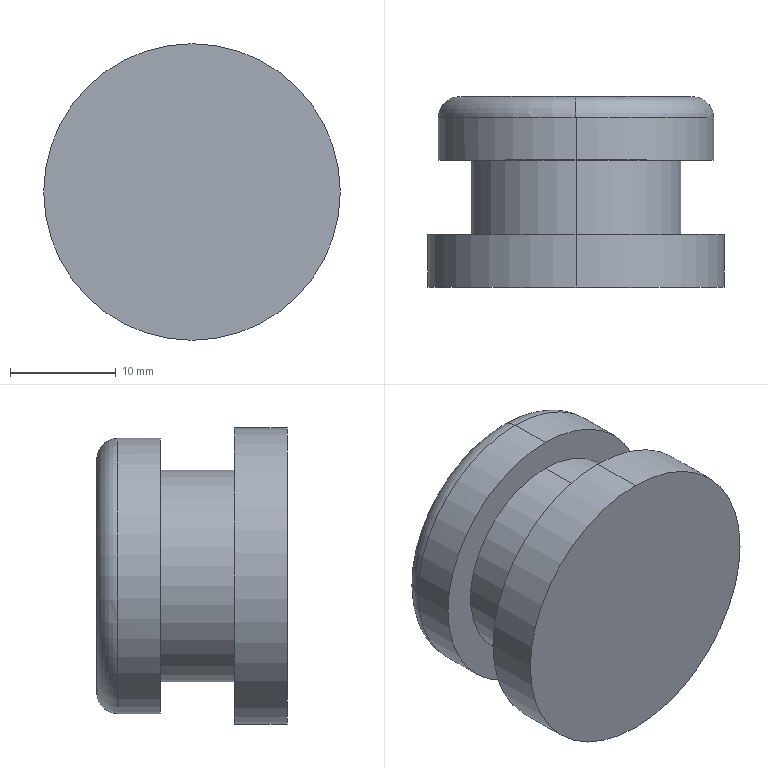Part | NX | features solid 2 | 1 solid | 12 faces | box 28 x 18 x 28 mm | volume 8396 mm3 | cylinder 6 | plane 4 | torus 2 | commonest cylinder face diameters 20 x2 26 x2 28 x2
STEP:
#1=CARTESIAN_POINT('',(-190.,-22.1,-151.));
#2=VERTEX_POINT('',#1);
#3=CARTESIAN_POINT('',(-190.,-22.1,-123.));
#4=VERTEX_POINT('',#3);
#5=CARTESIAN_POINT('',(-190.,-22.1,-137.));
#6=DIRECTION('',(0.,-1.,0.));
#7=DIRECTION('',(0.,0.,-1.));
#8=AXIS2_PLACEMENT_3D('',#5,#6,#7);
#9=CIRCLE('',#8,14.);
#10=EDGE_CURVE('',#2,#4,#9,.T.);
#11=ORIENTED_EDGE('',*,*,#10,.T.);
#12=CARTESIAN_POINT('',(-190.,-27.1,-123.));
#13=VERTEX_POINT('',#12);
#14=CARTESIAN_POINT('',(-190.,-27.1,-123.));
#15=DIRECTION('',(0.,1.,0.));
#16=VECTOR('',#15,1000.);
#17=LINE('',#14,#16);
#18=EDGE_CURVE('',#13,#4,#17,.T.);
#19=ORIENTED_EDGE('',*,*,#18,.F.);
#20=CARTESIAN_POINT('',(-190.,-27.1,-151.));
#21=VERTEX_POINT('',#20);
#22=CARTESIAN_POINT('',(-190.,-27.1,-137.));
#23=DIRECTION('',(0.,1.,0.));
#24=DIRECTION('',(0.,0.,1.));
#25=AXIS2_PLACEMENT_3D('',#22,#23,#24);
#26=CIRCLE('',#25,14.);
#27=EDGE_CURVE('',#13,#21,#26,.T.);
#28=ORIENTED_EDGE('',*,*,#27,.T.);
#29=CARTESIAN_POINT('',(-190.,-27.1,-151.));
#30=DIRECTION('',(0.,1.,0.));
#31=VECTOR('',#30,1000.);
#32=LINE('',#29,#31);
#33=EDGE_CURVE('',#2,#21,#32,.F.);
#34=ORIENTED_EDGE('',*,*,#33,.F.);
#35=EDGE_LOOP('',(#11,#19,#28,#34));
#36=FACE_BOUND('',#35,.T.);
#37=CARTESIAN_POINT('',(-190.,-21.85,-137.));
#38=DIRECTION('',(0.,-1.,0.));
#39=DIRECTION('',(0.,0.,-1.));
#40=AXIS2_PLACEMENT_3D('',#37,#38,#39);
#41=CYLINDRICAL_SURFACE('',#40,14.);
#42=ADVANCED_FACE('',(#36),#41,.T.);
#43=ORIENTED_EDGE('',*,*,#33,.T.);
#44=CARTESIAN_POINT('',(-190.,-27.1,-137.));
#45=DIRECTION('',(0.,1.,0.));
#46=DIRECTION('',(0.,0.,-1.));
#47=AXIS2_PLACEMENT_3D('',#44,#45,#46);
#48=CIRCLE('',#47,14.);
#49=EDGE_CURVE('',#21,#13,#48,.T.);
#50=ORIENTED_EDGE('',*,*,#49,.T.);
#51=ORIENTED_EDGE('',*,*,#18,.T.);
#52=CARTESIAN_POINT('',(-190.,-22.1,-137.));
#53=DIRECTION('',(0.,-1.,0.));
#54=DIRECTION('',(0.,0.,1.));
#55=AXIS2_PLACEMENT_3D('',#52,#53,#54);
#56=CIRCLE('',#55,14.);
#57=EDGE_CURVE('',#4,#2,#56,.T.);
#58=ORIENTED_EDGE('',*,*,#57,.T.);
#59=EDGE_LOOP('',(#43,#50,#51,#58));
#60=FACE_BOUND('',#59,.T.);
#61=CARTESIAN_POINT('',(-190.,-21.85,-137.));
#62=DIRECTION('',(0.,-1.,0.));
#63=DIRECTION('',(0.,0.,-1.));
#64=AXIS2_PLACEMENT_3D('',#61,#62,#63);
#65=CYLINDRICAL_SURFACE('',#64,14.);
#66=ADVANCED_FACE('',(#60),#65,.T.);
#67=ORIENTED_EDGE('',*,*,#10,.F.);
#68=ORIENTED_EDGE('',*,*,#57,.F.);
#69=EDGE_LOOP('',(#67,#68));
#70=FACE_BOUND('',#69,.T.);
#71=CARTESIAN_POINT('',(-190.,-22.1,-147.));
#72=VERTEX_POINT('',#71);
#73=CARTESIAN_POINT('',(-190.,-22.1,-127.));
#74=VERTEX_POINT('',#73);
#75=CARTESIAN_POINT('',(-190.,-22.1,-137.));
#76=DIRECTION('',(0.,1.,0.));
#77=DIRECTION('',(0.,0.,-1.));
#78=AXIS2_PLACEMENT_3D('',#75,#76,#77);
#79=CIRCLE('',#78,10.);
#80=EDGE_CURVE('',#72,#74,#79,.T.);
#81=ORIENTED_EDGE('',*,*,#80,.F.);
#82=CARTESIAN_POINT('',(-190.,-22.1,-137.));
#83=DIRECTION('',(0.,1.,0.));
#84=DIRECTION('',(0.,0.,1.));
#85=AXIS2_PLACEMENT_3D('',#82,#83,#84);
#86=CIRCLE('',#85,10.);
#87=EDGE_CURVE('',#74,#72,#86,.T.);
#88=ORIENTED_EDGE('',*,*,#87,.F.);
#89=EDGE_LOOP('',(#81,#88));
#90=FACE_BOUND('',#89,.T.);
#91=CARTESIAN_POINT('',(-190.,-22.1,-137.));
#92=DIRECTION('',(0.,-1.,0.));
#93=DIRECTION('',(0.,0.,-1.));
#94=AXIS2_PLACEMENT_3D('',#91,#92,#93);
#95=PLANE('',#94);
#96=ADVANCED_FACE('',(#70,#90),#95,.F.);
#97=CARTESIAN_POINT('',(-190.,-15.1,-147.));
#98=VERTEX_POINT('',#97);
#99=CARTESIAN_POINT('',(-190.,-15.1,-127.));
#100=VERTEX_POINT('',#99);
#101=CARTESIAN_POINT('',(-190.,-15.1,-137.));
#102=DIRECTION('',(0.,-1.,0.));
#103=DIRECTION('',(0.,0.,-1.));
#104=AXIS2_PLACEMENT_3D('',#101,#102,#103);
#105=CIRCLE('',#104,10.);
#106=EDGE_CURVE('',#98,#100,#105,.T.);
#107=ORIENTED_EDGE('',*,*,#106,.T.);
#108=CARTESIAN_POINT('',(-190.,-22.1,-127.));
#109=DIRECTION('',(0.,1.,0.));
#110=VECTOR('',#109,1000.);
#111=LINE('',#108,#110);
#112=EDGE_CURVE('',#100,#74,#111,.F.);
#113=ORIENTED_EDGE('',*,*,#112,.T.);
#114=ORIENTED_EDGE('',*,*,#87,.T.);
#115=CARTESIAN_POINT('',(-190.,-22.1,-147.));
#116=DIRECTION('',(0.,1.,0.));
#117=VECTOR('',#116,1000.);
#118=LINE('',#115,#117);
#119=EDGE_CURVE('',#72,#98,#118,.T.);
#120=ORIENTED_EDGE('',*,*,#119,.T.);
#121=EDGE_LOOP('',(#107,#113,#114,#120));
#122=FACE_BOUND('',#121,.T.);
#123=CARTESIAN_POINT('',(-190.,-15.1,-137.));
#124=DIRECTION('',(0.,-1.,0.));
#125=DIRECTION('',(0.,0.,-1.));
#126=AXIS2_PLACEMENT_3D('',#123,#124,#125);
#127=CYLINDRICAL_SURFACE('',#126,10.);
#128=ADVANCED_FACE('',(#122),#127,.T.);
#129=ORIENTED_EDGE('',*,*,#119,.F.);
#130=ORIENTED_EDGE('',*,*,#80,.T.);
#131=ORIENTED_EDGE('',*,*,#112,.F.);
#132=CARTESIAN_POINT('',(-190.,-15.1,-137.));
#133=DIRECTION('',(0.,-1.,0.));
#134=DIRECTION('',(0.,0.,1.));
#135=AXIS2_PLACEMENT_3D('',#132,#133,#134);
#136=CIRCLE('',#135,10.);
#137=EDGE_CURVE('',#100,#98,#136,.T.);
#138=ORIENTED_EDGE('',*,*,#137,.T.);
#139=EDGE_LOOP('',(#129,#130,#131,#138));
#140=FACE_BOUND('',#139,.T.);
#141=CARTESIAN_POINT('',(-190.,-15.1,-137.));
#142=DIRECTION('',(0.,-1.,0.));
#143=DIRECTION('',(0.,0.,-1.));
#144=AXIS2_PLACEMENT_3D('',#141,#142,#143);
#145=CYLINDRICAL_SURFACE('',#144,10.);
#146=ADVANCED_FACE('',(#140),#145,.T.);
#147=CARTESIAN_POINT('',(-190.,-15.1,-124.));
#148=VERTEX_POINT('',#147);
#149=CARTESIAN_POINT('',(-190.,-15.1,-150.));
#150=VERTEX_POINT('',#149);
#151=CARTESIAN_POINT('',(-190.,-15.1,-137.));
#152=DIRECTION('',(0.,1.,0.));
#153=DIRECTION('',(0.,0.,1.));
#154=AXIS2_PLACEMENT_3D('',#151,#152,#153);
#155=CIRCLE('',#154,13.);
#156=EDGE_CURVE('',#148,#150,#155,.T.);
#157=ORIENTED_EDGE('',*,*,#156,.F.);
#158=CARTESIAN_POINT('',(-190.,-15.1,-137.));
#159=DIRECTION('',(0.,1.,0.));
#160=DIRECTION('',(0.,0.,-1.));
#161=AXIS2_PLACEMENT_3D('',#158,#159,#160);
#162=CIRCLE('',#161,13.);
#163=EDGE_CURVE('',#150,#148,#162,.T.);
#164=ORIENTED_EDGE('',*,*,#163,.F.);
#165=EDGE_LOOP('',(#157,#164));
#166=FACE_BOUND('',#165,.T.);
#167=ORIENTED_EDGE('',*,*,#106,.F.);
#168=ORIENTED_EDGE('',*,*,#137,.F.);
#169=EDGE_LOOP('',(#167,#168));
#170=FACE_BOUND('',#169,.T.);
#171=CARTESIAN_POINT('',(-190.,-15.1,-137.));
#172=DIRECTION('',(0.,-1.,0.));
#173=DIRECTION('',(0.,0.,-1.));
#174=AXIS2_PLACEMENT_3D('',#171,#172,#173);
#175=PLANE('',#174);
#176=ADVANCED_FACE('',(#166,#170),#175,.T.);
#177=CARTESIAN_POINT('',(-190.089,-11.1,-124.));
#178=VERTEX_POINT('',#177);
#179=CARTESIAN_POINT('',(-190.,-11.1,-150.));
#180=VERTEX_POINT('',#179);
#181=CARTESIAN_POINT('',(-190.,-11.1,-137.));
#182=DIRECTION('',(0.,-1.,0.));
#183=DIRECTION('',(-0.006879,0.,1.));
#184=AXIS2_PLACEMENT_3D('',#181,#182,#183);
#185=CIRCLE('',#184,13.);
#186=EDGE_CURVE('',#178,#180,#185,.T.);
#187=ORIENTED_EDGE('',*,*,#186,.T.);
#188=CARTESIAN_POINT('',(-190.,-15.1,-150.));
#189=DIRECTION('',(0.,1.,0.));
#190=VECTOR('',#189,1000.);
#191=LINE('',#188,#190);
#192=EDGE_CURVE('',#180,#150,#191,.F.);
#193=ORIENTED_EDGE('',*,*,#192,.T.);
#194=ORIENTED_EDGE('',*,*,#163,.T.);
#195=CARTESIAN_POINT('',(-190.,-11.1,-124.));
#196=VERTEX_POINT('',#195);
#197=CARTESIAN_POINT('',(-190.,-15.1,-124.));
#198=DIRECTION('',(0.,1.,0.));
#199=VECTOR('',#198,1000.);
#200=LINE('',#197,#199);
#201=EDGE_CURVE('',#148,#196,#200,.T.);
#202=ORIENTED_EDGE('',*,*,#201,.T.);
#203=CARTESIAN_POINT('',(-190.,-11.1,-137.));
#204=DIRECTION('',(0.,-1.,0.));
#205=DIRECTION('',(0.,0.,1.));
#206=AXIS2_PLACEMENT_3D('',#203,#204,#205);
#207=CIRCLE('',#206,13.);
#208=EDGE_CURVE('',#196,#178,#207,.T.);
#209=ORIENTED_EDGE('',*,*,#208,.T.);
#210=EDGE_LOOP('',(#187,#193,#194,#202,#209));
#211=FACE_BOUND('',#210,.T.);
#212=CARTESIAN_POINT('',(-190.,-9.1,-137.));
#213=DIRECTION('',(0.,-1.,0.));
#214=DIRECTION('',(0.,0.,-1.));
#215=AXIS2_PLACEMENT_3D('',#212,#213,#214);
#216=CYLINDRICAL_SURFACE('',#215,13.);
#217=ADVANCED_FACE('',(#211),#216,.T.);
#218=ORIENTED_EDGE('',*,*,#208,.F.);
#219=CARTESIAN_POINT('',(-189.911,-11.1,-150.));
#220=VERTEX_POINT('',#219);
#221=CARTESIAN_POINT('',(-190.,-11.1,-137.));
#222=DIRECTION('',(0.,-1.,0.));
#223=DIRECTION('',(0.006879,0.,-1.));
#224=AXIS2_PLACEMENT_3D('',#221,#222,#223);
#225=CIRCLE('',#224,13.);
#226=EDGE_CURVE('',#220,#196,#225,.T.);
#227=ORIENTED_EDGE('',*,*,#226,.F.);
#228=CARTESIAN_POINT('',(-189.925,-9.1,-148.));
#229=VERTEX_POINT('',#228);
#230=CARTESIAN_POINT('',(-189.924,-11.1,-148.));
#231=DIRECTION('',(-1.,0.,-0.006879));
#232=DIRECTION('',(0.,1.,0.000000001));
#233=AXIS2_PLACEMENT_3D('',#230,#231,#232);
#234=CIRCLE('',#233,2.);
#235=EDGE_CURVE('',#220,#229,#234,.F.);
#236=ORIENTED_EDGE('',*,*,#235,.T.);
#237=CARTESIAN_POINT('',(-190.,-9.1,-126.));
#238=VERTEX_POINT('',#237);
#239=CARTESIAN_POINT('',(-190.,-9.1,-137.));
#240=DIRECTION('',(0.,-1.,0.));
#241=DIRECTION('',(0.006861,0.,-1.));
#242=AXIS2_PLACEMENT_3D('',#239,#240,#241);
#243=CIRCLE('',#242,11.);
#244=EDGE_CURVE('',#229,#238,#243,.T.);
#245=ORIENTED_EDGE('',*,*,#244,.T.);
#246=CARTESIAN_POINT('',(-190.076,-9.1,-126.));
#247=VERTEX_POINT('',#246);
#248=CARTESIAN_POINT('',(-190.,-9.1,-137.));
#249=DIRECTION('',(0.,1.,0.));
#250=DIRECTION('',(-0.006944,0.,1.));
#251=AXIS2_PLACEMENT_3D('',#248,#249,#250);
#252=CIRCLE('',#251,11.);
#253=EDGE_CURVE('',#238,#247,#252,.F.);
#254=ORIENTED_EDGE('',*,*,#253,.T.);
#255=CARTESIAN_POINT('',(-190.076,-11.1,-126.));
#256=DIRECTION('',(1.,0.,0.006879));
#257=DIRECTION('',(0.,1.,-0.000000001));
#258=AXIS2_PLACEMENT_3D('',#255,#256,#257);
#259=CIRCLE('',#258,2.);
#260=EDGE_CURVE('',#247,#178,#259,.T.);
#261=ORIENTED_EDGE('',*,*,#260,.T.);
#262=EDGE_LOOP('',(#218,#227,#236,#245,#254,#261));
#263=FACE_BOUND('',#262,.T.);
#264=CARTESIAN_POINT('',(-190.,-11.1,-137.));
#265=DIRECTION('',(0.,1.,0.));
#266=DIRECTION('',(-0.006879,0.,1.));
#267=AXIS2_PLACEMENT_3D('',#264,#265,#266);
#268=TOROIDAL_SURFACE('',#267,11.,2.);
#269=ADVANCED_FACE('',(#263),#268,.T.);
#270=ORIENTED_EDGE('',*,*,#260,.F.);
#271=CARTESIAN_POINT('',(-190.,-9.1,-148.));
#272=VERTEX_POINT('',#271);
#273=CARTESIAN_POINT('',(-190.,-9.1,-137.));
#274=DIRECTION('',(0.,-1.,0.));
#275=DIRECTION('',(-0.006944,0.,1.));
#276=AXIS2_PLACEMENT_3D('',#273,#274,#275);
#277=CIRCLE('',#276,11.);
#278=EDGE_CURVE('',#247,#272,#277,.T.);
#279=ORIENTED_EDGE('',*,*,#278,.T.);
#280=CARTESIAN_POINT('',(-190.,-9.1,-137.));
#281=DIRECTION('',(0.,1.,0.));
#282=DIRECTION('',(0.006861,0.,-1.));
#283=AXIS2_PLACEMENT_3D('',#280,#281,#282);
#284=CIRCLE('',#283,11.);
#285=EDGE_CURVE('',#272,#229,#284,.F.);
#286=ORIENTED_EDGE('',*,*,#285,.T.);
#287=ORIENTED_EDGE('',*,*,#235,.F.);
#288=CARTESIAN_POINT('',(-190.,-11.1,-137.));
#289=DIRECTION('',(0.,-1.,0.));
#290=DIRECTION('',(0.,0.,-1.));
#291=AXIS2_PLACEMENT_3D('',#288,#289,#290);
#292=CIRCLE('',#291,13.);
#293=EDGE_CURVE('',#180,#220,#292,.T.);
#294=ORIENTED_EDGE('',*,*,#293,.F.);
#295=ORIENTED_EDGE('',*,*,#186,.F.);
#296=EDGE_LOOP('',(#270,#279,#286,#287,#294,#295));
#297=FACE_BOUND('',#296,.T.);
#298=CARTESIAN_POINT('',(-190.,-11.1,-137.));
#299=DIRECTION('',(0.,1.,0.));
#300=DIRECTION('',(0.006879,0.,-1.));
#301=AXIS2_PLACEMENT_3D('',#298,#299,#300);
#302=TOROIDAL_SURFACE('',#301,11.,2.);
#303=ADVANCED_FACE('',(#297),#302,.T.);
#304=ORIENTED_EDGE('',*,*,#293,.T.);
#305=ORIENTED_EDGE('',*,*,#226,.T.);
#306=ORIENTED_EDGE('',*,*,#201,.F.);
#307=ORIENTED_EDGE('',*,*,#156,.T.);
#308=ORIENTED_EDGE('',*,*,#192,.F.);
#309=EDGE_LOOP('',(#304,#305,#306,#307,#308));
#310=FACE_BOUND('',#309,.T.);
#311=CARTESIAN_POINT('',(-190.,-9.1,-137.));
#312=DIRECTION('',(0.,-1.,0.));
#313=DIRECTION('',(0.,0.,-1.));
#314=AXIS2_PLACEMENT_3D('',#311,#312,#313);
#315=CYLINDRICAL_SURFACE('',#314,13.);
#316=ADVANCED_FACE('',(#310),#315,.T.);
#317=ORIENTED_EDGE('',*,*,#244,.F.);
#318=ORIENTED_EDGE('',*,*,#285,.F.);
#319=ORIENTED_EDGE('',*,*,#278,.F.);
#320=ORIENTED_EDGE('',*,*,#253,.F.);
#321=EDGE_LOOP('',(#317,#318,#319,#320));
#322=FACE_BOUND('',#321,.T.);
#323=CARTESIAN_POINT('',(-190.,-9.1,-137.));
#324=DIRECTION('',(0.,-1.,0.));
#325=DIRECTION('',(0.,0.,-1.));
#326=AXIS2_PLACEMENT_3D('',#323,#324,#325);
#327=PLANE('',#326);
#328=ADVANCED_FACE('',(#322),#327,.F.);
#329=ORIENTED_EDGE('',*,*,#27,.F.);
#330=ORIENTED_EDGE('',*,*,#49,.F.);
#331=EDGE_LOOP('',(#329,#330));
#332=FACE_BOUND('',#331,.T.);
#333=CARTESIAN_POINT('',(-190.,-27.1,-137.));
#334=DIRECTION('',(0.,-1.,0.));
#335=DIRECTION('',(0.,0.,-1.));
#336=AXIS2_PLACEMENT_3D('',#333,#334,#335);
#337=PLANE('',#336);
#338=ADVANCED_FACE('',(#332),#337,.T.);
#339=CLOSED_SHELL('',(#42,#66,#96,#128,#146,#176,#217,#269,#303,#316,#328,#338));
#340=MANIFOLD_SOLID_BREP('',#339);
#341=(LENGTH_UNIT()NAMED_UNIT(*)SI_UNIT(.MILLI.,.METRE.));
#342=UNCERTAINTY_MEASURE_WITH_UNIT(LENGTH_MEASURE(0.00001),#341,'','');
#343=(NAMED_UNIT(*)PLANE_ANGLE_UNIT()SI_UNIT($,.RADIAN.));
#344=(NAMED_UNIT(*)SI_UNIT($,.STERADIAN.)SOLID_ANGLE_UNIT());
#345=(GEOMETRIC_REPRESENTATION_CONTEXT(3)GLOBAL_UNCERTAINTY_ASSIGNED_CONTEXT((#342))GLOBAL_UNIT_ASSIGNED_CONTEXT((#341,#343,#344))REPRESENTATION_CONTEXT('',''));
#346=ADVANCED_BREP_SHAPE_REPRESENTATION('',(#340),#345);